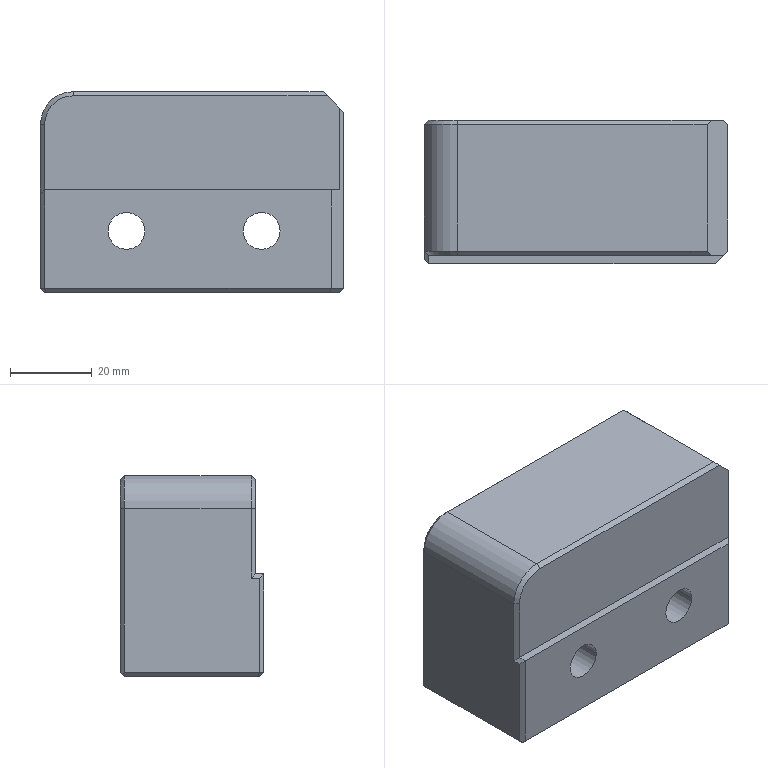Part | Creo | 1 solid | 36 faces | box 74 x 35 x 49 mm | volume 116048 mm3 | plane 25 | cylinder 9 | cone 2 | commonest cylinder face diameters 9 x4 14 x4 16 x1
STEP:
#1=CARTESIAN_POINT('',(-133.,331.995,-295.));
#2=VERTEX_POINT('',#1);
#3=CARTESIAN_POINT('',(-133.,331.995,-271.));
#4=VERTEX_POINT('',#3);
#5=CARTESIAN_POINT('',(-133.,331.995,-295.));
#6=DIRECTION('',(0.,0.,1.));
#7=VECTOR('',#6,24.);
#8=LINE('',#5,#7);
#9=EDGE_CURVE('',#2,#4,#8,.T.);
#10=ORIENTED_EDGE('',*,*,#9,.T.);
#11=CARTESIAN_POINT('',(-63.,331.995,-271.));
#12=VERTEX_POINT('',#11);
#13=CARTESIAN_POINT('',(-133.,331.995,-271.));
#14=DIRECTION('',(1.,0.,0.));
#15=VECTOR('',#14,70.);
#16=LINE('',#13,#15);
#17=EDGE_CURVE('',#4,#12,#16,.T.);
#18=ORIENTED_EDGE('',*,*,#17,.T.);
#19=CARTESIAN_POINT('',(-63.,331.995,-295.));
#20=VERTEX_POINT('',#19);
#21=CARTESIAN_POINT('',(-63.,331.995,-271.));
#22=DIRECTION('',(0.,0.,-1.));
#23=VECTOR('',#22,24.);
#24=LINE('',#21,#23);
#25=EDGE_CURVE('',#12,#20,#24,.T.);
#26=ORIENTED_EDGE('',*,*,#25,.T.);
#27=CARTESIAN_POINT('',(-63.,331.995,-295.));
#28=DIRECTION('',(-1.,0.,0.));
#29=VECTOR('',#28,70.);
#30=LINE('',#27,#29);
#31=EDGE_CURVE('',#20,#2,#30,.T.);
#32=ORIENTED_EDGE('',*,*,#31,.T.);
#33=EDGE_LOOP('',(#10,#18,#26,#32));
#34=FACE_OUTER_BOUND('',#33,.F.);
#35=CARTESIAN_POINT('',(-108.5,331.995,-281.));
#36=VERTEX_POINT('',#35);
#37=CARTESIAN_POINT('',(-117.5,331.995,-281.));
#38=VERTEX_POINT('',#37);
#39=CARTESIAN_POINT('',(-113.,331.995,-281.));
#40=DIRECTION('',(0.,1.,0.));
#41=DIRECTION('',(1.,0.,0.));
#42=AXIS2_PLACEMENT_3D('',#39,#40,#41);
#43=CIRCLE('',#42,4.5);
#44=EDGE_CURVE('',#36,#38,#43,.T.);
#45=ORIENTED_EDGE('',*,*,#44,.F.);
#46=CARTESIAN_POINT('',(-113.,331.995,-281.));
#47=DIRECTION('',(0.,1.,0.));
#48=DIRECTION('',(-1.,0.,0.));
#49=AXIS2_PLACEMENT_3D('',#46,#47,#48);
#50=CIRCLE('',#49,4.5);
#51=EDGE_CURVE('',#38,#36,#50,.T.);
#52=ORIENTED_EDGE('',*,*,#51,.F.);
#53=EDGE_LOOP('',(#45,#52));
#54=FACE_BOUND('',#53,.F.);
#55=CARTESIAN_POINT('',(-75.5,331.995,-281.));
#56=VERTEX_POINT('',#55);
#57=CARTESIAN_POINT('',(-84.5,331.995,-281.));
#58=VERTEX_POINT('',#57);
#59=CARTESIAN_POINT('',(-80.,331.995,-281.));
#60=DIRECTION('',(0.,1.,0.));
#61=DIRECTION('',(1.,0.,0.));
#62=AXIS2_PLACEMENT_3D('',#59,#60,#61);
#63=CIRCLE('',#62,4.5);
#64=EDGE_CURVE('',#56,#58,#63,.T.);
#65=ORIENTED_EDGE('',*,*,#64,.F.);
#66=CARTESIAN_POINT('',(-80.,331.995,-281.));
#67=DIRECTION('',(0.,1.,0.));
#68=DIRECTION('',(-1.,0.,0.));
#69=AXIS2_PLACEMENT_3D('',#66,#67,#68);
#70=CIRCLE('',#69,4.5);
#71=EDGE_CURVE('',#58,#56,#70,.T.);
#72=ORIENTED_EDGE('',*,*,#71,.F.);
#73=EDGE_LOOP('',(#65,#72));
#74=FACE_BOUND('',#73,.F.);
#75=CARTESIAN_POINT('',(-162.,331.995,-10.));
#76=DIRECTION('',(0.,1.,0.));
#77=DIRECTION('',(-1.,0.,0.));
#78=AXIS2_PLACEMENT_3D('',#75,#76,#77);
#79=PLANE('',#78);
#80=ADVANCED_FACE('',(#34,#54,#74),#79,.F.);
#81=ORIENTED_EDGE('',*,*,#64,.T.);
#82=CARTESIAN_POINT('',(-84.5,357.995,-281.));
#83=VERTEX_POINT('',#82);
#84=CARTESIAN_POINT('',(-84.5,331.995,-281.));
#85=DIRECTION('',(0.,1.,0.));
#86=VECTOR('',#85,26.);
#87=LINE('',#84,#86);
#88=EDGE_CURVE('',#58,#83,#87,.T.);
#89=ORIENTED_EDGE('',*,*,#88,.T.);
#90=CARTESIAN_POINT('',(-75.5,357.995,-281.));
#91=VERTEX_POINT('',#90);
#92=CARTESIAN_POINT('',(-80.,357.995,-281.));
#93=DIRECTION('',(0.,-1.,0.));
#94=DIRECTION('',(-1.,0.,0.));
#95=AXIS2_PLACEMENT_3D('',#92,#93,#94);
#96=CIRCLE('',#95,4.5);
#97=EDGE_CURVE('',#83,#91,#96,.T.);
#98=ORIENTED_EDGE('',*,*,#97,.T.);
#99=CARTESIAN_POINT('',(-75.5,331.995,-281.));
#100=DIRECTION('',(0.,1.,0.));
#101=VECTOR('',#100,26.);
#102=LINE('',#99,#101);
#103=EDGE_CURVE('',#56,#91,#102,.T.);
#104=ORIENTED_EDGE('',*,*,#103,.F.);
#105=EDGE_LOOP('',(#81,#89,#98,#104));
#106=FACE_OUTER_BOUND('',#105,.F.);
#107=CARTESIAN_POINT('',(-80.,366.995,-281.));
#108=DIRECTION('',(0.,1.,0.));
#109=DIRECTION('',(-1.,0.,0.));
#110=AXIS2_PLACEMENT_3D('',#107,#108,#109);
#111=CYLINDRICAL_SURFACE('',#110,4.5);
#112=ADVANCED_FACE('',(#106),#111,.F.);
#113=ORIENTED_EDGE('',*,*,#71,.T.);
#114=ORIENTED_EDGE('',*,*,#103,.T.);
#115=CARTESIAN_POINT('',(-80.,357.995,-281.));
#116=DIRECTION('',(0.,-1.,0.));
#117=DIRECTION('',(1.,0.,0.));
#118=AXIS2_PLACEMENT_3D('',#115,#116,#117);
#119=CIRCLE('',#118,4.5);
#120=EDGE_CURVE('',#91,#83,#119,.T.);
#121=ORIENTED_EDGE('',*,*,#120,.T.);
#122=ORIENTED_EDGE('',*,*,#88,.F.);
#123=EDGE_LOOP('',(#113,#114,#121,#122));
#124=FACE_OUTER_BOUND('',#123,.F.);
#125=CARTESIAN_POINT('',(-80.,366.995,-281.));
#126=DIRECTION('',(0.,1.,0.));
#127=DIRECTION('',(-1.,0.,0.));
#128=AXIS2_PLACEMENT_3D('',#125,#126,#127);
#129=CYLINDRICAL_SURFACE('',#128,4.5);
#130=ADVANCED_FACE('',(#124),#129,.F.);
#131=CARTESIAN_POINT('',(-73.,357.995,-281.));
#132=VERTEX_POINT('',#131);
#133=CARTESIAN_POINT('',(-87.,357.995,-281.));
#134=VERTEX_POINT('',#133);
#135=CARTESIAN_POINT('',(-80.,357.995,-281.));
#136=DIRECTION('',(0.,1.,0.));
#137=DIRECTION('',(1.,0.,0.));
#138=AXIS2_PLACEMENT_3D('',#135,#136,#137);
#139=CIRCLE('',#138,7.);
#140=EDGE_CURVE('',#132,#134,#139,.T.);
#141=ORIENTED_EDGE('',*,*,#140,.F.);
#142=CARTESIAN_POINT('',(-80.,357.995,-281.));
#143=DIRECTION('',(0.,1.,0.));
#144=DIRECTION('',(-1.,0.,0.));
#145=AXIS2_PLACEMENT_3D('',#142,#143,#144);
#146=CIRCLE('',#145,7.);
#147=EDGE_CURVE('',#134,#132,#146,.T.);
#148=ORIENTED_EDGE('',*,*,#147,.F.);
#149=EDGE_LOOP('',(#141,#148));
#150=FACE_OUTER_BOUND('',#149,.F.);
#151=ORIENTED_EDGE('',*,*,#120,.F.);
#152=ORIENTED_EDGE('',*,*,#97,.F.);
#153=EDGE_LOOP('',(#151,#152));
#154=FACE_BOUND('',#153,.F.);
#155=CARTESIAN_POINT('',(-80.,357.995,-288.));
#156=DIRECTION('',(0.,-1.,0.));
#157=DIRECTION('',(1.,0.,0.));
#158=AXIS2_PLACEMENT_3D('',#155,#156,#157);
#159=PLANE('',#158);
#160=ADVANCED_FACE('',(#150,#154),#159,.F.);
#161=ORIENTED_EDGE('',*,*,#140,.T.);
#162=CARTESIAN_POINT('',(-87.,366.995,-281.));
#163=VERTEX_POINT('',#162);
#164=CARTESIAN_POINT('',(-87.,357.995,-281.));
#165=DIRECTION('',(0.,1.,0.));
#166=VECTOR('',#165,9.);
#167=LINE('',#164,#166);
#168=EDGE_CURVE('',#134,#163,#167,.T.);
#169=ORIENTED_EDGE('',*,*,#168,.T.);
#170=CARTESIAN_POINT('',(-73.,366.995,-281.));
#171=VERTEX_POINT('',#170);
#172=CARTESIAN_POINT('',(-80.,366.995,-281.));
#173=DIRECTION('',(0.,-1.,0.));
#174=DIRECTION('',(-1.,0.,0.));
#175=AXIS2_PLACEMENT_3D('',#172,#173,#174);
#176=CIRCLE('',#175,7.);
#177=EDGE_CURVE('',#163,#171,#176,.T.);
#178=ORIENTED_EDGE('',*,*,#177,.T.);
#179=CARTESIAN_POINT('',(-73.,357.995,-281.));
#180=DIRECTION('',(0.,1.,0.));
#181=VECTOR('',#180,9.);
#182=LINE('',#179,#181);
#183=EDGE_CURVE('',#132,#171,#182,.T.);
#184=ORIENTED_EDGE('',*,*,#183,.F.);
#185=EDGE_LOOP('',(#161,#169,#178,#184));
#186=FACE_OUTER_BOUND('',#185,.F.);
#187=CARTESIAN_POINT('',(-80.,366.995,-281.));
#188=DIRECTION('',(0.,1.,0.));
#189=DIRECTION('',(-1.,0.,0.));
#190=AXIS2_PLACEMENT_3D('',#187,#188,#189);
#191=CYLINDRICAL_SURFACE('',#190,7.);
#192=ADVANCED_FACE('',(#186),#191,.F.);
#193=ORIENTED_EDGE('',*,*,#147,.T.);
#194=ORIENTED_EDGE('',*,*,#183,.T.);
#195=CARTESIAN_POINT('',(-80.,366.995,-281.));
#196=DIRECTION('',(0.,-1.,0.));
#197=DIRECTION('',(1.,0.,0.));
#198=AXIS2_PLACEMENT_3D('',#195,#196,#197);
#199=CIRCLE('',#198,7.);
#200=EDGE_CURVE('',#171,#163,#199,.T.);
#201=ORIENTED_EDGE('',*,*,#200,.T.);
#202=ORIENTED_EDGE('',*,*,#168,.F.);
#203=EDGE_LOOP('',(#193,#194,#201,#202));
#204=FACE_OUTER_BOUND('',#203,.F.);
#205=CARTESIAN_POINT('',(-80.,366.995,-281.));
#206=DIRECTION('',(0.,1.,0.));
#207=DIRECTION('',(-1.,0.,0.));
#208=AXIS2_PLACEMENT_3D('',#205,#206,#207);
#209=CYLINDRICAL_SURFACE('',#208,7.);
#210=ADVANCED_FACE('',(#204),#209,.F.);
#211=CARTESIAN_POINT('',(-64.,366.995,-248.));
#212=VERTEX_POINT('',#211);
#213=CARTESIAN_POINT('',(-126.,366.995,-248.));
#214=VERTEX_POINT('',#213);
#215=CARTESIAN_POINT('',(-64.,366.995,-248.));
#216=DIRECTION('',(-1.,0.,0.));
#217=VECTOR('',#216,62.);
#218=LINE('',#215,#217);
#219=EDGE_CURVE('',#212,#214,#218,.T.);
#220=ORIENTED_EDGE('',*,*,#219,.T.);
#221=CARTESIAN_POINT('',(-133.,366.995,-255.));
#222=VERTEX_POINT('',#221);
#223=CARTESIAN_POINT('',(-126.,366.995,-255.));
#224=DIRECTION('',(0.,1.,0.));
#225=DIRECTION('',(-1.,0.,0.));
#226=AXIS2_PLACEMENT_3D('',#223,#224,#225);
#227=CIRCLE('',#226,7.);
#228=EDGE_CURVE('',#222,#214,#227,.T.);
#229=ORIENTED_EDGE('',*,*,#228,.F.);
#230=CARTESIAN_POINT('',(-133.,366.995,-295.));
#231=VERTEX_POINT('',#230);
#232=CARTESIAN_POINT('',(-133.,366.995,-255.));
#233=DIRECTION('',(0.,0.,-1.));
#234=VECTOR('',#233,40.);
#235=LINE('',#232,#234);
#236=EDGE_CURVE('',#222,#231,#235,.T.);
#237=ORIENTED_EDGE('',*,*,#236,.T.);
#238=CARTESIAN_POINT('',(-61.,366.995,-295.));
#239=VERTEX_POINT('',#238);
#240=CARTESIAN_POINT('',(-133.,366.995,-295.));
#241=DIRECTION('',(1.,0.,0.));
#242=VECTOR('',#241,72.);
#243=LINE('',#240,#242);
#244=EDGE_CURVE('',#231,#239,#243,.T.);
#245=ORIENTED_EDGE('',*,*,#244,.T.);
#246=CARTESIAN_POINT('',(-61.,366.995,-251.));
#247=VERTEX_POINT('',#246);
#248=CARTESIAN_POINT('',(-61.,366.995,-295.));
#249=DIRECTION('',(0.,0.,1.));
#250=VECTOR('',#249,44.);
#251=LINE('',#248,#250);
#252=EDGE_CURVE('',#239,#247,#251,.T.);
#253=ORIENTED_EDGE('',*,*,#252,.T.);
#254=CARTESIAN_POINT('',(-64.,366.995,-248.));
#255=DIRECTION('',(0.7071,0.,-0.7071));
#256=VECTOR('',#255,4.243);
#257=LINE('',#254,#256);
#258=EDGE_CURVE('',#212,#247,#257,.T.);
#259=ORIENTED_EDGE('',*,*,#258,.F.);
#260=EDGE_LOOP('',(#220,#229,#237,#245,#253,#259));
#261=FACE_OUTER_BOUND('',#260,.F.);
#262=CARTESIAN_POINT('',(-106.,366.995,-281.));
#263=VERTEX_POINT('',#262);
#264=CARTESIAN_POINT('',(-120.,366.995,-281.));
#265=VERTEX_POINT('',#264);
#266=CARTESIAN_POINT('',(-113.,366.995,-281.));
#267=DIRECTION('',(0.,-1.,0.));
#268=DIRECTION('',(1.,0.,0.));
#269=AXIS2_PLACEMENT_3D('',#266,#267,#268);
#270=CIRCLE('',#269,7.);
#271=EDGE_CURVE('',#263,#265,#270,.T.);
#272=ORIENTED_EDGE('',*,*,#271,.F.);
#273=CARTESIAN_POINT('',(-113.,366.995,-281.));
#274=DIRECTION('',(0.,-1.,0.));
#275=DIRECTION('',(-1.,0.,0.));
#276=AXIS2_PLACEMENT_3D('',#273,#274,#275);
#277=CIRCLE('',#276,7.);
#278=EDGE_CURVE('',#265,#263,#277,.T.);
#279=ORIENTED_EDGE('',*,*,#278,.F.);
#280=EDGE_LOOP('',(#272,#279));
#281=FACE_BOUND('',#280,.F.);
#282=ORIENTED_EDGE('',*,*,#200,.F.);
#283=ORIENTED_EDGE('',*,*,#177,.F.);
#284=EDGE_LOOP('',(#282,#283));
#285=FACE_BOUND('',#284,.F.);
#286=CARTESIAN_POINT('',(-162.,366.995,-10.));
#287=DIRECTION('',(0.,1.,0.));
#288=DIRECTION('',(-1.,0.,0.));
#289=AXIS2_PLACEMENT_3D('',#286,#287,#288);
#290=PLANE('',#289);
#291=ADVANCED_FACE('',(#261,#281,#285),#290,.T.);
#292=CARTESIAN_POINT('',(-120.,357.995,-281.));
#293=VERTEX_POINT('',#292);
#294=CARTESIAN_POINT('',(-106.,357.995,-281.));
#295=VERTEX_POINT('',#294);
#296=CARTESIAN_POINT('',(-113.,357.995,-281.));
#297=DIRECTION('',(0.,1.,0.));
#298=DIRECTION('',(-1.,0.,0.));
#299=AXIS2_PLACEMENT_3D('',#296,#297,#298);
#300=CIRCLE('',#299,7.);
#301=EDGE_CURVE('',#293,#295,#300,.T.);
#302=ORIENTED_EDGE('',*,*,#301,.T.);
#303=CARTESIAN_POINT('',(-106.,357.995,-281.));
#304=DIRECTION('',(0.,1.,0.));
#305=VECTOR('',#304,9.);
#306=LINE('',#303,#305);
#307=EDGE_CURVE('',#295,#263,#306,.T.);
#308=ORIENTED_EDGE('',*,*,#307,.T.);
#309=ORIENTED_EDGE('',*,*,#271,.T.);
#310=CARTESIAN_POINT('',(-120.,357.995,-281.));
#311=DIRECTION('',(0.,1.,0.));
#312=VECTOR('',#311,9.);
#313=LINE('',#310,#312);
#314=EDGE_CURVE('',#293,#265,#313,.T.);
#315=ORIENTED_EDGE('',*,*,#314,.F.);
#316=EDGE_LOOP('',(#302,#308,#309,#315));
#317=FACE_OUTER_BOUND('',#316,.F.);
#318=CARTESIAN_POINT('',(-113.,366.995,-281.));
#319=DIRECTION('',(0.,1.,0.));
#320=DIRECTION('',(-1.,0.,0.));
#321=AXIS2_PLACEMENT_3D('',#318,#319,#320);
#322=CYLINDRICAL_SURFACE('',#321,7.);
#323=ADVANCED_FACE('',(#317),#322,.F.);
#324=CARTESIAN_POINT('',(-113.,357.995,-281.));
#325=DIRECTION('',(0.,1.,0.));
#326=DIRECTION('',(1.,0.,0.));
#327=AXIS2_PLACEMENT_3D('',#324,#325,#326);
#328=CIRCLE('',#327,7.);
#329=EDGE_CURVE('',#295,#293,#328,.T.);
#330=ORIENTED_EDGE('',*,*,#329,.F.);
#331=ORIENTED_EDGE('',*,*,#301,.F.);
#332=EDGE_LOOP('',(#330,#331));
#333=FACE_OUTER_BOUND('',#332,.F.);
#334=CARTESIAN_POINT('',(-108.5,357.995,-281.));
#335=VERTEX_POINT('',#334);
#336=CARTESIAN_POINT('',(-117.5,357.995,-281.));
#337=VERTEX_POINT('',#336);
#338=CARTESIAN_POINT('',(-113.,357.995,-281.));
#339=DIRECTION('',(0.,-1.,0.));
#340=DIRECTION('',(1.,0.,0.));
#341=AXIS2_PLACEMENT_3D('',#338,#339,#340);
#342=CIRCLE('',#341,4.5);
#343=EDGE_CURVE('',#335,#337,#342,.T.);
#344=ORIENTED_EDGE('',*,*,#343,.F.);
#345=CARTESIAN_POINT('',(-113.,357.995,-281.));
#346=DIRECTION('',(0.,-1.,0.));
#347=DIRECTION('',(-1.,0.,0.));
#348=AXIS2_PLACEMENT_3D('',#345,#346,#347);
#349=CIRCLE('',#348,4.5);
#350=EDGE_CURVE('',#337,#335,#349,.T.);
#351=ORIENTED_EDGE('',*,*,#350,.F.);
#352=EDGE_LOOP('',(#344,#351));
#353=FACE_BOUND('',#352,.F.);
#354=CARTESIAN_POINT('',(-113.,357.995,-288.));
#355=DIRECTION('',(0.,-1.,0.));
#356=DIRECTION('',(1.,0.,0.));
#357=AXIS2_PLACEMENT_3D('',#354,#355,#356);
#358=PLANE('',#357);
#359=ADVANCED_FACE('',(#333,#353),#358,.F.);
#360=ORIENTED_EDGE('',*,*,#51,.T.);
#361=CARTESIAN_POINT('',(-108.5,331.995,-281.));
#362=DIRECTION('',(0.,1.,0.));
#363=VECTOR('',#362,26.);
#364=LINE('',#361,#363);
#365=EDGE_CURVE('',#36,#335,#364,.T.);
#366=ORIENTED_EDGE('',*,*,#365,.T.);
#367=ORIENTED_EDGE('',*,*,#343,.T.);
#368=CARTESIAN_POINT('',(-117.5,331.995,-281.));
#369=DIRECTION('',(0.,1.,0.));
#370=VECTOR('',#369,26.);
#371=LINE('',#368,#370);
#372=EDGE_CURVE('',#38,#337,#371,.T.);
#373=ORIENTED_EDGE('',*,*,#372,.F.);
#374=EDGE_LOOP('',(#360,#366,#367,#373));
#375=FACE_OUTER_BOUND('',#374,.F.);
#376=CARTESIAN_POINT('',(-113.,366.995,-281.));
#377=DIRECTION('',(0.,1.,0.));
#378=DIRECTION('',(-1.,0.,0.));
#379=AXIS2_PLACEMENT_3D('',#376,#377,#378);
#380=CYLINDRICAL_SURFACE('',#379,4.5);
#381=ADVANCED_FACE('',(#375),#380,.F.);
#382=ORIENTED_EDGE('',*,*,#44,.T.);
#383=ORIENTED_EDGE('',*,*,#372,.T.);
#384=ORIENTED_EDGE('',*,*,#350,.T.);
#385=ORIENTED_EDGE('',*,*,#365,.F.);
#386=EDGE_LOOP('',(#382,#383,#384,#385));
#387=FACE_OUTER_BOUND('',#386,.F.);
#388=CARTESIAN_POINT('',(-113.,366.995,-281.));
#389=DIRECTION('',(0.,1.,0.));
#390=DIRECTION('',(-1.,0.,0.));
#391=AXIS2_PLACEMENT_3D('',#388,#389,#390);
#392=CYLINDRICAL_SURFACE('',#391,4.5);
#393=ADVANCED_FACE('',(#387),#392,.F.);
#394=ORIENTED_EDGE('',*,*,#329,.T.);
#395=ORIENTED_EDGE('',*,*,#314,.T.);
#396=ORIENTED_EDGE('',*,*,#278,.T.);
#397=ORIENTED_EDGE('',*,*,#307,.F.);
#398=EDGE_LOOP('',(#394,#395,#396,#397));
#399=FACE_OUTER_BOUND('',#398,.F.);
#400=CARTESIAN_POINT('',(-113.,366.995,-281.));
#401=DIRECTION('',(0.,1.,0.));
#402=DIRECTION('',(-1.,0.,0.));
#403=AXIS2_PLACEMENT_3D('',#400,#401,#402);
#404=CYLINDRICAL_SURFACE('',#403,7.);
#405=ADVANCED_FACE('',(#399),#404,.F.);
#406=CARTESIAN_POINT('',(-65.,365.995,-247.));
#407=VERTEX_POINT('',#406);
#408=CARTESIAN_POINT('',(-126.,365.995,-247.));
#409=VERTEX_POINT('',#408);
#410=CARTESIAN_POINT('',(-65.,365.995,-247.));
#411=DIRECTION('',(-1.,0.,0.));
#412=VECTOR('',#411,61.);
#413=LINE('',#410,#412);
#414=EDGE_CURVE('',#407,#409,#413,.T.);
#415=ORIENTED_EDGE('',*,*,#414,.T.);
#416=CARTESIAN_POINT('',(-126.,365.995,-247.));
#417=DIRECTION('',(0.,0.7071,-0.7071));
#418=VECTOR('',#417,1.414);
#419=LINE('',#416,#418);
#420=EDGE_CURVE('',#409,#214,#419,.T.);
#421=ORIENTED_EDGE('',*,*,#420,.T.);
#422=ORIENTED_EDGE('',*,*,#219,.F.);
#423=CARTESIAN_POINT('',(-64.,366.995,-248.));
#424=DIRECTION('',(-0.5774,-0.5774,0.5774));
#425=VECTOR('',#424,1.732);
#426=LINE('',#423,#425);
#427=EDGE_CURVE('',#212,#407,#426,.T.);
#428=ORIENTED_EDGE('',*,*,#427,.T.);
#429=EDGE_LOOP('',(#415,#421,#422,#428));
#430=FACE_OUTER_BOUND('',#429,.F.);
#431=CARTESIAN_POINT('',(-112.,366.495,-247.5));
#432=DIRECTION('',(0.,0.7071,0.7071));
#433=DIRECTION('',(0.,-0.7071,0.7071));
#434=AXIS2_PLACEMENT_3D('',#431,#432,#433);
#435=PLANE('',#434);
#436=ADVANCED_FACE('',(#430),#435,.T.);
#437=CARTESIAN_POINT('',(-65.,334.995,-247.));
#438=VERTEX_POINT('',#437);
#439=CARTESIAN_POINT('',(-126.,334.995,-247.));
#440=VERTEX_POINT('',#439);
#441=CARTESIAN_POINT('',(-65.,334.995,-247.));
#442=DIRECTION('',(-1.,0.,0.));
#443=VECTOR('',#442,61.);
#444=LINE('',#441,#443);
#445=EDGE_CURVE('',#438,#440,#444,.T.);
#446=ORIENTED_EDGE('',*,*,#445,.T.);
#447=CARTESIAN_POINT('',(-126.,334.995,-247.));
#448=DIRECTION('',(0.,1.,0.));
#449=VECTOR('',#448,31.);
#450=LINE('',#447,#449);
#451=EDGE_CURVE('',#440,#409,#450,.T.);
#452=ORIENTED_EDGE('',*,*,#451,.T.);
#453=ORIENTED_EDGE('',*,*,#414,.F.);
#454=CARTESIAN_POINT('',(-65.,365.995,-247.));
#455=DIRECTION('',(0.,-1.,0.));
#456=VECTOR('',#455,31.);
#457=LINE('',#454,#456);
#458=EDGE_CURVE('',#407,#438,#457,.T.);
#459=ORIENTED_EDGE('',*,*,#458,.T.);
#460=EDGE_LOOP('',(#446,#452,#453,#459));
#461=FACE_OUTER_BOUND('',#460,.F.);
#462=CARTESIAN_POINT('',(-135.,331.995,-247.));
#463=DIRECTION('',(0.,0.,1.));
#464=DIRECTION('',(1.,0.,0.));
#465=AXIS2_PLACEMENT_3D('',#462,#463,#464);
#466=PLANE('',#465);
#467=ADVANCED_FACE('',(#461),#466,.T.);
#468=CARTESIAN_POINT('',(-64.,333.995,-248.));
#469=VERTEX_POINT('',#468);
#470=CARTESIAN_POINT('',(-126.,333.995,-248.));
#471=VERTEX_POINT('',#470);
#472=CARTESIAN_POINT('',(-64.,333.995,-248.));
#473=DIRECTION('',(-1.,0.,0.));
#474=VECTOR('',#473,62.);
#475=LINE('',#472,#474);
#476=EDGE_CURVE('',#469,#471,#475,.T.);
#477=ORIENTED_EDGE('',*,*,#476,.T.);
#478=CARTESIAN_POINT('',(-126.,333.995,-248.));
#479=DIRECTION('',(0.,0.7071,0.7071));
#480=VECTOR('',#479,1.414);
#481=LINE('',#478,#480);
#482=EDGE_CURVE('',#471,#440,#481,.T.);
#483=ORIENTED_EDGE('',*,*,#482,.T.);
#484=ORIENTED_EDGE('',*,*,#445,.F.);
#485=CARTESIAN_POINT('',(-65.,334.995,-247.));
#486=DIRECTION('',(0.5774,-0.5774,-0.5774));
#487=VECTOR('',#486,1.732);
#488=LINE('',#485,#487);
#489=EDGE_CURVE('',#438,#469,#488,.T.);
#490=ORIENTED_EDGE('',*,*,#489,.T.);
#491=EDGE_LOOP('',(#477,#483,#484,#490));
#492=FACE_OUTER_BOUND('',#491,.F.);
#493=CARTESIAN_POINT('',(-112.,334.495,-247.5));
#494=DIRECTION('',(0.,-0.7071,0.7071));
#495=DIRECTION('',(0.,-0.7071,-0.7071));
#496=AXIS2_PLACEMENT_3D('',#493,#494,#495);
#497=PLANE('',#496);
#498=ADVANCED_FACE('',(#492),#497,.T.);
#499=CARTESIAN_POINT('',(-61.,333.995,-251.));
#500=VERTEX_POINT('',#499);
#501=CARTESIAN_POINT('',(-61.,333.995,-271.));
#502=VERTEX_POINT('',#501);
#503=CARTESIAN_POINT('',(-61.,333.995,-251.));
#504=DIRECTION('',(0.,0.,-1.));
#505=VECTOR('',#504,20.);
#506=LINE('',#503,#505);
#507=EDGE_CURVE('',#500,#502,#506,.T.);
#508=ORIENTED_EDGE('',*,*,#507,.T.);
#509=CARTESIAN_POINT('',(-133.,333.995,-271.));
#510=VERTEX_POINT('',#509);
#511=CARTESIAN_POINT('',(-61.,333.995,-271.));
#512=DIRECTION('',(-1.,0.,0.));
#513=VECTOR('',#512,72.);
#514=LINE('',#511,#513);
#515=EDGE_CURVE('',#502,#510,#514,.T.);
#516=ORIENTED_EDGE('',*,*,#515,.T.);
#517=CARTESIAN_POINT('',(-133.,333.995,-255.));
#518=VERTEX_POINT('',#517);
#519=CARTESIAN_POINT('',(-133.,333.995,-255.));
#520=DIRECTION('',(0.,0.,-1.));
#521=VECTOR('',#520,16.);
#522=LINE('',#519,#521);
#523=EDGE_CURVE('',#518,#510,#522,.T.);
#524=ORIENTED_EDGE('',*,*,#523,.F.);
#525=CARTESIAN_POINT('',(-126.,333.995,-255.));
#526=DIRECTION('',(0.,-1.,0.));
#527=DIRECTION('',(0.,0.,1.));
#528=AXIS2_PLACEMENT_3D('',#525,#526,#527);
#529=CIRCLE('',#528,7.);
#530=EDGE_CURVE('',#471,#518,#529,.T.);
#531=ORIENTED_EDGE('',*,*,#530,.F.);
#532=ORIENTED_EDGE('',*,*,#476,.F.);
#533=CARTESIAN_POINT('',(-61.,333.995,-251.));
#534=DIRECTION('',(-0.7071,0.,0.7071));
#535=VECTOR('',#534,4.243);
#536=LINE('',#533,#535);
#537=EDGE_CURVE('',#500,#469,#536,.T.);
#538=ORIENTED_EDGE('',*,*,#537,.F.);
#539=EDGE_LOOP('',(#508,#516,#524,#531,#532,#538));
#540=FACE_OUTER_BOUND('',#539,.F.);
#541=CARTESIAN_POINT('',(-162.,333.995,-10.));
#542=DIRECTION('',(0.,-1.,0.));
#543=DIRECTION('',(1.,0.,0.));
#544=AXIS2_PLACEMENT_3D('',#541,#542,#543);
#545=PLANE('',#544);
#546=ADVANCED_FACE('',(#540),#545,.T.);
#547=ORIENTED_EDGE('',*,*,#25,.F.);
#548=CARTESIAN_POINT('',(-63.,331.995,-271.));
#549=DIRECTION('',(0.7071,0.7071,0.));
#550=VECTOR('',#549,2.828);
#551=LINE('',#548,#550);
#552=EDGE_CURVE('',#12,#502,#551,.T.);
#553=ORIENTED_EDGE('',*,*,#552,.T.);
#554=ORIENTED_EDGE('',*,*,#507,.F.);
#555=CARTESIAN_POINT('',(-60.,334.995,-252.));
#556=VERTEX_POINT('',#555);
#557=CARTESIAN_POINT('',(-61.,333.995,-251.));
#558=DIRECTION('',(0.5774,0.5774,-0.5774));
#559=VECTOR('',#558,1.732);
#560=LINE('',#557,#559);
#561=EDGE_CURVE('',#500,#556,#560,.T.);
#562=ORIENTED_EDGE('',*,*,#561,.T.);
#563=CARTESIAN_POINT('',(-60.,334.995,-295.));
#564=VERTEX_POINT('',#563);
#565=CARTESIAN_POINT('',(-60.,334.995,-295.));
#566=DIRECTION('',(0.,0.,1.));
#567=VECTOR('',#566,43.);
#568=LINE('',#565,#567);
#569=EDGE_CURVE('',#564,#556,#568,.T.);
#570=ORIENTED_EDGE('',*,*,#569,.F.);
#571=CARTESIAN_POINT('',(-60.,334.995,-295.));
#572=DIRECTION('',(-0.7071,-0.7071,0.));
#573=VECTOR('',#572,4.243);
#574=LINE('',#571,#573);
#575=EDGE_CURVE('',#564,#20,#574,.T.);
#576=ORIENTED_EDGE('',*,*,#575,.T.);
#577=EDGE_LOOP('',(#547,#553,#554,#562,#570,#576));
#578=FACE_OUTER_BOUND('',#577,.F.);
#579=CARTESIAN_POINT('',(-63.,331.995,-10.));
#580=DIRECTION('',(0.7071,-0.7071,0.));
#581=DIRECTION('',(0.,0.,1.));
#582=AXIS2_PLACEMENT_3D('',#579,#580,#581);
#583=PLANE('',#582);
#584=ADVANCED_FACE('',(#578),#583,.T.);
#585=ORIENTED_EDGE('',*,*,#17,.F.);
#586=CARTESIAN_POINT('',(-133.,333.995,-271.));
#587=DIRECTION('',(0.,-1.,0.));
#588=VECTOR('',#587,2.);
#589=LINE('',#586,#588);
#590=EDGE_CURVE('',#510,#4,#589,.T.);
#591=ORIENTED_EDGE('',*,*,#590,.F.);
#592=ORIENTED_EDGE('',*,*,#515,.F.);
#593=ORIENTED_EDGE('',*,*,#552,.F.);
#594=EDGE_LOOP('',(#585,#591,#592,#593));
#595=FACE_OUTER_BOUND('',#594,.F.);
#596=CARTESIAN_POINT('',(-227.861,331.995,-271.));
#597=DIRECTION('',(0.,0.,-1.));
#598=DIRECTION('',(1.,0.,0.));
#599=AXIS2_PLACEMENT_3D('',#596,#597,#598);
#600=PLANE('',#599);
#601=ADVANCED_FACE('',(#595),#600,.F.);
#602=ORIENTED_EDGE('',*,*,#590,.T.);
#603=CARTESIAN_POINT('',(-134.,332.995,-272.));
#604=VERTEX_POINT('',#603);
#605=CARTESIAN_POINT('',(-134.,332.995,-272.));
#606=DIRECTION('',(0.5774,-0.5774,0.5774));
#607=VECTOR('',#606,1.732);
#608=LINE('',#605,#607);
#609=EDGE_CURVE('',#604,#4,#608,.T.);
#610=ORIENTED_EDGE('',*,*,#609,.F.);
#611=CARTESIAN_POINT('',(-134.,334.995,-272.));
#612=VERTEX_POINT('',#611);
#613=CARTESIAN_POINT('',(-134.,334.995,-272.));
#614=DIRECTION('',(0.,-1.,0.));
#615=VECTOR('',#614,2.);
#616=LINE('',#613,#615);
#617=EDGE_CURVE('',#612,#604,#616,.T.);
#618=ORIENTED_EDGE('',*,*,#617,.F.);
#619=CARTESIAN_POINT('',(-134.,334.995,-272.));
#620=DIRECTION('',(0.5774,-0.5774,0.5774));
#621=VECTOR('',#620,1.732);
#622=LINE('',#619,#621);
#623=EDGE_CURVE('',#612,#510,#622,.T.);
#624=ORIENTED_EDGE('',*,*,#623,.T.);
#625=EDGE_LOOP('',(#602,#610,#618,#624));
#626=FACE_OUTER_BOUND('',#625,.F.);
#627=CARTESIAN_POINT('',(-133.5,333.495,-271.5));
#628=DIRECTION('',(-0.7071,0.,0.7071));
#629=DIRECTION('',(0.7071,0.,0.7071));
#630=AXIS2_PLACEMENT_3D('',#627,#628,#629);
#631=PLANE('',#630);
#632=ADVANCED_FACE('',(#626),#631,.T.);
#633=CARTESIAN_POINT('',(-134.,332.995,-295.));
#634=VERTEX_POINT('',#633);
#635=CARTESIAN_POINT('',(-134.,332.995,-295.));
#636=DIRECTION('',(0.,0.,1.));
#637=VECTOR('',#636,23.);
#638=LINE('',#635,#637);
#639=EDGE_CURVE('',#634,#604,#638,.T.);
#640=ORIENTED_EDGE('',*,*,#639,.T.);
#641=ORIENTED_EDGE('',*,*,#609,.T.);
#642=ORIENTED_EDGE('',*,*,#9,.F.);
#643=CARTESIAN_POINT('',(-133.,331.995,-295.));
#644=DIRECTION('',(-0.7071,0.7071,0.));
#645=VECTOR('',#644,1.414);
#646=LINE('',#643,#645);
#647=EDGE_CURVE('',#2,#634,#646,.T.);
#648=ORIENTED_EDGE('',*,*,#647,.T.);
#649=EDGE_LOOP('',(#640,#641,#642,#648));
#650=FACE_OUTER_BOUND('',#649,.F.);
#651=CARTESIAN_POINT('',(-133.5,332.495,-289.));
#652=DIRECTION('',(-0.7071,-0.7071,0.));
#653=DIRECTION('',(-0.7071,0.7071,0.));
#654=AXIS2_PLACEMENT_3D('',#651,#652,#653);
#655=PLANE('',#654);
#656=ADVANCED_FACE('',(#650),#655,.T.);
#657=CARTESIAN_POINT('',(-134.,365.995,-255.));
#658=VERTEX_POINT('',#657);
#659=CARTESIAN_POINT('',(-134.,365.995,-295.));
#660=VERTEX_POINT('',#659);
#661=CARTESIAN_POINT('',(-134.,365.995,-255.));
#662=DIRECTION('',(0.,0.,-1.));
#663=VECTOR('',#662,40.);
#664=LINE('',#661,#663);
#665=EDGE_CURVE('',#658,#660,#664,.T.);
#666=ORIENTED_EDGE('',*,*,#665,.F.);
#667=CARTESIAN_POINT('',(-134.,334.995,-255.));
#668=VERTEX_POINT('',#667);
#669=CARTESIAN_POINT('',(-134.,365.995,-255.));
#670=DIRECTION('',(0.,-1.,0.));
#671=VECTOR('',#670,31.);
#672=LINE('',#669,#671);
#673=EDGE_CURVE('',#658,#668,#672,.T.);
#674=ORIENTED_EDGE('',*,*,#673,.T.);
#675=CARTESIAN_POINT('',(-134.,334.995,-255.));
#676=DIRECTION('',(0.,0.,-1.));
#677=VECTOR('',#676,17.);
#678=LINE('',#675,#677);
#679=EDGE_CURVE('',#668,#612,#678,.T.);
#680=ORIENTED_EDGE('',*,*,#679,.T.);
#681=ORIENTED_EDGE('',*,*,#617,.T.);
#682=ORIENTED_EDGE('',*,*,#639,.F.);
#683=CARTESIAN_POINT('',(-134.,332.995,-295.));
#684=DIRECTION('',(0.,1.,0.));
#685=VECTOR('',#684,33.);
#686=LINE('',#683,#685);
#687=EDGE_CURVE('',#634,#660,#686,.T.);
#688=ORIENTED_EDGE('',*,*,#687,.T.);
#689=EDGE_LOOP('',(#666,#674,#680,#681,#682,#688));
#690=FACE_OUTER_BOUND('',#689,.F.);
#691=CARTESIAN_POINT('',(-134.,331.995,-326.));
#692=DIRECTION('',(-1.,0.,0.));
#693=DIRECTION('',(0.,0.,1.));
#694=AXIS2_PLACEMENT_3D('',#691,#692,#693);
#695=PLANE('',#694);
#696=ADVANCED_FACE('',(#690),#695,.T.);
#697=CARTESIAN_POINT('',(-133.5,366.495,-295.5));
#698=VERTEX_POINT('',#697);
#699=CARTESIAN_POINT('',(-133.5,366.495,-295.5));
#700=DIRECTION('',(0.5774,0.5774,0.5774));
#701=VECTOR('',#700,0.866);
#702=LINE('',#699,#701);
#703=EDGE_CURVE('',#698,#231,#702,.T.);
#704=ORIENTED_EDGE('',*,*,#703,.T.);
#705=ORIENTED_EDGE('',*,*,#236,.F.);
#706=CARTESIAN_POINT('',(-133.,366.995,-255.));
#707=DIRECTION('',(-0.7071,-0.7071,0.));
#708=VECTOR('',#707,1.414);
#709=LINE('',#706,#708);
#710=EDGE_CURVE('',#222,#658,#709,.T.);
#711=ORIENTED_EDGE('',*,*,#710,.T.);
#712=ORIENTED_EDGE('',*,*,#665,.T.);
#713=CARTESIAN_POINT('',(-134.,365.995,-295.));
#714=DIRECTION('',(0.5774,0.5774,-0.5774));
#715=VECTOR('',#714,0.866);
#716=LINE('',#713,#715);
#717=EDGE_CURVE('',#660,#698,#716,.T.);
#718=ORIENTED_EDGE('',*,*,#717,.T.);
#719=EDGE_LOOP('',(#704,#705,#711,#712,#718));
#720=FACE_OUTER_BOUND('',#719,.F.);
#721=CARTESIAN_POINT('',(-133.5,366.495,-289.));
#722=DIRECTION('',(-0.7071,0.7071,0.));
#723=DIRECTION('',(-0.7071,-0.7071,0.));
#724=AXIS2_PLACEMENT_3D('',#721,#722,#723);
#725=PLANE('',#724);
#726=ADVANCED_FACE('',(#720),#725,.T.);
#727=CARTESIAN_POINT('',(-60.5,366.495,-295.5));
#728=VERTEX_POINT('',#727);
#729=CARTESIAN_POINT('',(-60.5,366.495,-295.5));
#730=DIRECTION('',(-0.5774,0.5774,0.5774));
#731=VECTOR('',#730,0.866);
#732=LINE('',#729,#731);
#733=EDGE_CURVE('',#728,#239,#732,.T.);
#734=ORIENTED_EDGE('',*,*,#733,.T.);
#735=ORIENTED_EDGE('',*,*,#244,.F.);
#736=ORIENTED_EDGE('',*,*,#703,.F.);
#737=CARTESIAN_POINT('',(-133.,365.995,-296.));
#738=VERTEX_POINT('',#737);
#739=CARTESIAN_POINT('',(-133.5,366.495,-295.5));
#740=DIRECTION('',(0.5774,-0.5774,-0.5774));
#741=VECTOR('',#740,0.866);
#742=LINE('',#739,#741);
#743=EDGE_CURVE('',#698,#738,#742,.T.);
#744=ORIENTED_EDGE('',*,*,#743,.T.);
#745=CARTESIAN_POINT('',(-61.,365.995,-296.));
#746=VERTEX_POINT('',#745);
#747=CARTESIAN_POINT('',(-61.,365.995,-296.));
#748=DIRECTION('',(-1.,0.,0.));
#749=VECTOR('',#748,72.);
#750=LINE('',#747,#749);
#751=EDGE_CURVE('',#746,#738,#750,.T.);
#752=ORIENTED_EDGE('',*,*,#751,.F.);
#753=CARTESIAN_POINT('',(-61.,365.995,-296.));
#754=DIRECTION('',(0.5774,0.5774,0.5774));
#755=VECTOR('',#754,0.866);
#756=LINE('',#753,#755);
#757=EDGE_CURVE('',#746,#728,#756,.T.);
#758=ORIENTED_EDGE('',*,*,#757,.T.);
#759=EDGE_LOOP('',(#734,#735,#736,#744,#752,#758));
#760=FACE_OUTER_BOUND('',#759,.F.);
#761=CARTESIAN_POINT('',(-110.5,365.995,-296.));
#762=DIRECTION('',(0.,0.7071,-0.7071));
#763=DIRECTION('',(1.,0.,0.));
#764=AXIS2_PLACEMENT_3D('',#761,#762,#763);
#765=PLANE('',#764);
#766=ADVANCED_FACE('',(#760),#765,.T.);
#767=CARTESIAN_POINT('',(-60.,365.995,-252.));
#768=VERTEX_POINT('',#767);
#769=CARTESIAN_POINT('',(-60.,365.995,-295.));
#770=VERTEX_POINT('',#769);
#771=CARTESIAN_POINT('',(-60.,365.995,-252.));
#772=DIRECTION('',(0.,0.,-1.));
#773=VECTOR('',#772,43.);
#774=LINE('',#771,#773);
#775=EDGE_CURVE('',#768,#770,#774,.T.);
#776=ORIENTED_EDGE('',*,*,#775,.F.);
#777=CARTESIAN_POINT('',(-60.,365.995,-252.));
#778=DIRECTION('',(-0.5774,0.5774,0.5774));
#779=VECTOR('',#778,1.732);
#780=LINE('',#777,#779);
#781=EDGE_CURVE('',#768,#247,#780,.T.);
#782=ORIENTED_EDGE('',*,*,#781,.T.);
#783=ORIENTED_EDGE('',*,*,#252,.F.);
#784=ORIENTED_EDGE('',*,*,#733,.F.);
#785=CARTESIAN_POINT('',(-60.5,366.495,-295.5));
#786=DIRECTION('',(0.5774,-0.5774,0.5774));
#787=VECTOR('',#786,0.866);
#788=LINE('',#785,#787);
#789=EDGE_CURVE('',#728,#770,#788,.T.);
#790=ORIENTED_EDGE('',*,*,#789,.T.);
#791=EDGE_LOOP('',(#776,#782,#783,#784,#790));
#792=FACE_OUTER_BOUND('',#791,.F.);
#793=CARTESIAN_POINT('',(-60.,365.995,-326.));
#794=DIRECTION('',(-0.7071,-0.7071,0.));
#795=DIRECTION('',(0.,0.,-1.));
#796=AXIS2_PLACEMENT_3D('',#793,#794,#795);
#797=PLANE('',#796);
#798=ADVANCED_FACE('',(#792),#797,.F.);
#799=ORIENTED_EDGE('',*,*,#569,.T.);
#800=CARTESIAN_POINT('',(-60.,334.995,-252.));
#801=DIRECTION('',(0.,1.,0.));
#802=VECTOR('',#801,31.);
#803=LINE('',#800,#802);
#804=EDGE_CURVE('',#556,#768,#803,.T.);
#805=ORIENTED_EDGE('',*,*,#804,.T.);
#806=ORIENTED_EDGE('',*,*,#775,.T.);
#807=CARTESIAN_POINT('',(-60.,365.995,-295.));
#808=DIRECTION('',(0.,-1.,0.));
#809=VECTOR('',#808,31.);
#810=LINE('',#807,#809);
#811=EDGE_CURVE('',#770,#564,#810,.T.);
#812=ORIENTED_EDGE('',*,*,#811,.T.);
#813=EDGE_LOOP('',(#799,#805,#806,#812));
#814=FACE_OUTER_BOUND('',#813,.F.);
#815=CARTESIAN_POINT('',(-60.,349.495,-326.));
#816=DIRECTION('',(1.,0.,0.));
#817=DIRECTION('',(0.,0.,-1.));
#818=AXIS2_PLACEMENT_3D('',#815,#816,#817);
#819=PLANE('',#818);
#820=ADVANCED_FACE('',(#814),#819,.T.);
#821=ORIENTED_EDGE('',*,*,#427,.F.);
#822=ORIENTED_EDGE('',*,*,#258,.T.);
#823=ORIENTED_EDGE('',*,*,#781,.F.);
#824=ORIENTED_EDGE('',*,*,#804,.F.);
#825=ORIENTED_EDGE('',*,*,#561,.F.);
#826=ORIENTED_EDGE('',*,*,#537,.T.);
#827=ORIENTED_EDGE('',*,*,#489,.F.);
#828=ORIENTED_EDGE('',*,*,#458,.F.);
#829=EDGE_LOOP('',(#821,#822,#823,#824,#825,#826,#827,#828));
#830=FACE_OUTER_BOUND('',#829,.F.);
#831=CARTESIAN_POINT('',(-60.,349.495,-252.));
#832=DIRECTION('',(-0.7071,0.,-0.7071));
#833=DIRECTION('',(0.,1.,0.));
#834=AXIS2_PLACEMENT_3D('',#831,#832,#833);
#835=PLANE('',#834);
#836=ADVANCED_FACE('',(#830),#835,.F.);
#837=CARTESIAN_POINT('',(-61.,335.41,-296.));
#838=VERTEX_POINT('',#837);
#839=CARTESIAN_POINT('',(-61.,335.41,-296.));
#840=DIRECTION('',(0.6786,-0.2811,0.6786));
#841=VECTOR('',#840,1.474);
#842=LINE('',#839,#841);
#843=EDGE_CURVE('',#838,#564,#842,.T.);
#844=ORIENTED_EDGE('',*,*,#843,.T.);
#845=ORIENTED_EDGE('',*,*,#811,.F.);
#846=ORIENTED_EDGE('',*,*,#789,.F.);
#847=ORIENTED_EDGE('',*,*,#757,.F.);
#848=CARTESIAN_POINT('',(-61.,335.41,-296.));
#849=DIRECTION('',(0.,1.,0.));
#850=VECTOR('',#849,30.586);
#851=LINE('',#848,#850);
#852=EDGE_CURVE('',#838,#746,#851,.T.);
#853=ORIENTED_EDGE('',*,*,#852,.F.);
#854=EDGE_LOOP('',(#844,#845,#846,#847,#853));
#855=FACE_OUTER_BOUND('',#854,.F.);
#856=CARTESIAN_POINT('',(-60.,349.495,-295.));
#857=DIRECTION('',(0.7071,0.,-0.7071));
#858=DIRECTION('',(0.,1.,0.));
#859=AXIS2_PLACEMENT_3D('',#856,#857,#858);
#860=PLANE('',#859);
#861=ADVANCED_FACE('',(#855),#860,.T.);
#862=CARTESIAN_POINT('',(-63.414,332.995,-296.));
#863=VERTEX_POINT('',#862);
#864=CARTESIAN_POINT('',(-63.414,332.995,-296.));
#865=DIRECTION('',(0.2811,-0.6786,0.6786));
#866=VECTOR('',#865,1.474);
#867=LINE('',#864,#866);
#868=EDGE_CURVE('',#863,#20,#867,.T.);
#869=ORIENTED_EDGE('',*,*,#868,.T.);
#870=ORIENTED_EDGE('',*,*,#575,.F.);
#871=ORIENTED_EDGE('',*,*,#843,.F.);
#872=CARTESIAN_POINT('',(-61.,335.41,-296.));
#873=DIRECTION('',(-0.7071,-0.7071,0.));
#874=VECTOR('',#873,3.414);
#875=LINE('',#872,#874);
#876=EDGE_CURVE('',#838,#863,#875,.T.);
#877=ORIENTED_EDGE('',*,*,#876,.T.);
#878=EDGE_LOOP('',(#869,#870,#871,#877));
#879=FACE_OUTER_BOUND('',#878,.F.);
#880=CARTESIAN_POINT('',(-78.707,317.702,-296.));
#881=DIRECTION('',(0.5,-0.5,-0.7071));
#882=DIRECTION('',(-0.7071,-0.7071,0.));
#883=AXIS2_PLACEMENT_3D('',#880,#881,#882);
#884=PLANE('',#883);
#885=ADVANCED_FACE('',(#879),#884,.T.);
#886=CARTESIAN_POINT('',(-132.586,332.995,-296.));
#887=VERTEX_POINT('',#886);
#888=CARTESIAN_POINT('',(-132.586,332.995,-296.));
#889=DIRECTION('',(-0.2811,-0.6786,0.6786));
#890=VECTOR('',#889,1.474);
#891=LINE('',#888,#890);
#892=EDGE_CURVE('',#887,#2,#891,.T.);
#893=ORIENTED_EDGE('',*,*,#892,.T.);
#894=ORIENTED_EDGE('',*,*,#31,.F.);
#895=ORIENTED_EDGE('',*,*,#868,.F.);
#896=CARTESIAN_POINT('',(-132.586,332.995,-296.));
#897=DIRECTION('',(1.,0.,0.));
#898=VECTOR('',#897,69.172);
#899=LINE('',#896,#898);
#900=EDGE_CURVE('',#887,#863,#899,.T.);
#901=ORIENTED_EDGE('',*,*,#900,.F.);
#902=EDGE_LOOP('',(#893,#894,#895,#901));
#903=FACE_OUTER_BOUND('',#902,.F.);
#904=CARTESIAN_POINT('',(-110.5,332.995,-296.));
#905=DIRECTION('',(0.,0.7071,0.7071));
#906=DIRECTION('',(1.,0.,0.));
#907=AXIS2_PLACEMENT_3D('',#904,#905,#906);
#908=PLANE('',#907);
#909=ADVANCED_FACE('',(#903),#908,.F.);
#910=CARTESIAN_POINT('',(-133.,333.41,-296.));
#911=VERTEX_POINT('',#910);
#912=CARTESIAN_POINT('',(-133.,333.41,-296.));
#913=DIRECTION('',(-0.6786,-0.2811,0.6786));
#914=VECTOR('',#913,1.474);
#915=LINE('',#912,#914);
#916=EDGE_CURVE('',#911,#634,#915,.T.);
#917=ORIENTED_EDGE('',*,*,#916,.T.);
#918=ORIENTED_EDGE('',*,*,#647,.F.);
#919=ORIENTED_EDGE('',*,*,#892,.F.);
#920=CARTESIAN_POINT('',(-132.586,332.995,-296.));
#921=DIRECTION('',(-0.7071,0.7071,0.));
#922=VECTOR('',#921,0.5858);
#923=LINE('',#920,#922);
#924=EDGE_CURVE('',#887,#911,#923,.T.);
#925=ORIENTED_EDGE('',*,*,#924,.T.);
#926=EDGE_LOOP('',(#917,#918,#919,#925));
#927=FACE_OUTER_BOUND('',#926,.F.);
#928=CARTESIAN_POINT('',(-129.293,329.702,-296.));
#929=DIRECTION('',(-0.5,-0.5,-0.7071));
#930=DIRECTION('',(-0.7071,0.7071,0.));
#931=AXIS2_PLACEMENT_3D('',#928,#929,#930);
#932=PLANE('',#931);
#933=ADVANCED_FACE('',(#927),#932,.T.);
#934=ORIENTED_EDGE('',*,*,#743,.F.);
#935=ORIENTED_EDGE('',*,*,#717,.F.);
#936=ORIENTED_EDGE('',*,*,#687,.F.);
#937=ORIENTED_EDGE('',*,*,#916,.F.);
#938=CARTESIAN_POINT('',(-133.,365.995,-296.));
#939=DIRECTION('',(0.,-1.,0.));
#940=VECTOR('',#939,32.586);
#941=LINE('',#938,#940);
#942=EDGE_CURVE('',#738,#911,#941,.T.);
#943=ORIENTED_EDGE('',*,*,#942,.F.);
#944=EDGE_LOOP('',(#934,#935,#936,#937,#943));
#945=FACE_OUTER_BOUND('',#944,.F.);
#946=CARTESIAN_POINT('',(-133.,349.495,-296.));
#947=DIRECTION('',(-0.7071,0.,-0.7071));
#948=DIRECTION('',(0.,1.,0.));
#949=AXIS2_PLACEMENT_3D('',#946,#947,#948);
#950=PLANE('',#949);
#951=ADVANCED_FACE('',(#945),#950,.T.);
#952=ORIENTED_EDGE('',*,*,#751,.T.);
#953=ORIENTED_EDGE('',*,*,#942,.T.);
#954=ORIENTED_EDGE('',*,*,#924,.F.);
#955=ORIENTED_EDGE('',*,*,#900,.T.);
#956=ORIENTED_EDGE('',*,*,#876,.F.);
#957=ORIENTED_EDGE('',*,*,#852,.T.);
#958=EDGE_LOOP('',(#952,#953,#954,#955,#956,#957));
#959=FACE_OUTER_BOUND('',#958,.F.);
#960=CARTESIAN_POINT('',(-110.5,349.495,-296.));
#961=DIRECTION('',(0.,0.,1.));
#962=DIRECTION('',(1.,0.,0.));
#963=AXIS2_PLACEMENT_3D('',#960,#961,#962);
#964=PLANE('',#963);
#965=ADVANCED_FACE('',(#959),#964,.F.);
#966=ORIENTED_EDGE('',*,*,#710,.F.);
#967=ORIENTED_EDGE('',*,*,#228,.T.);
#968=ORIENTED_EDGE('',*,*,#420,.F.);
#969=CARTESIAN_POINT('',(-126.,365.995,-255.));
#970=DIRECTION('',(0.,1.,0.));
#971=DIRECTION('',(-1.,0.,0.));
#972=AXIS2_PLACEMENT_3D('',#969,#970,#971);
#973=CIRCLE('',#972,8.);
#974=EDGE_CURVE('',#658,#409,#973,.T.);
#975=ORIENTED_EDGE('',*,*,#974,.F.);
#976=EDGE_LOOP('',(#966,#967,#968,#975));
#977=FACE_OUTER_BOUND('',#976,.F.);
#978=CARTESIAN_POINT('',(-126.,366.495,-255.));
#979=DIRECTION('',(0.,-1.,0.));
#980=DIRECTION('',(0.,0.,-1.));
#981=AXIS2_PLACEMENT_3D('',#978,#979,#980);
#982=CONICAL_SURFACE('',#981,7.5,45.);
#983=ADVANCED_FACE('',(#977),#982,.T.);
#984=ORIENTED_EDGE('',*,*,#451,.F.);
#985=CARTESIAN_POINT('',(-126.,334.995,-255.));
#986=DIRECTION('',(0.,-1.,0.));
#987=DIRECTION('',(0.,0.,1.));
#988=AXIS2_PLACEMENT_3D('',#985,#986,#987);
#989=CIRCLE('',#988,8.);
#990=EDGE_CURVE('',#440,#668,#989,.T.);
#991=ORIENTED_EDGE('',*,*,#990,.T.);
#992=ORIENTED_EDGE('',*,*,#673,.F.);
#993=ORIENTED_EDGE('',*,*,#974,.T.);
#994=EDGE_LOOP('',(#984,#991,#992,#993));
#995=FACE_OUTER_BOUND('',#994,.F.);
#996=CARTESIAN_POINT('',(-126.,412.621,-255.));
#997=DIRECTION('',(0.,-1.,0.));
#998=DIRECTION('',(0.,0.,1.));
#999=AXIS2_PLACEMENT_3D('',#996,#997,#998);
#1000=CYLINDRICAL_SURFACE('',#999,8.);
#1001=ADVANCED_FACE('',(#995),#1000,.T.);
#1002=CARTESIAN_POINT('',(-134.,334.995,-255.));
#1003=DIRECTION('',(0.7071,-0.7071,0.));
#1004=VECTOR('',#1003,1.414);
#1005=LINE('',#1002,#1004);
#1006=EDGE_CURVE('',#668,#518,#1005,.T.);
#1007=ORIENTED_EDGE('',*,*,#1006,.F.);
#1008=ORIENTED_EDGE('',*,*,#990,.F.);
#1009=ORIENTED_EDGE('',*,*,#482,.F.);
#1010=ORIENTED_EDGE('',*,*,#530,.T.);
#1011=EDGE_LOOP('',(#1007,#1008,#1009,#1010));
#1012=FACE_OUTER_BOUND('',#1011,.F.);
#1013=CARTESIAN_POINT('',(-126.,334.495,-255.));
#1014=DIRECTION('',(0.,1.,0.));
#1015=DIRECTION('',(0.,0.,-1.));
#1016=AXIS2_PLACEMENT_3D('',#1013,#1014,#1015);
#1017=CONICAL_SURFACE('',#1016,7.5,45.);
#1018=ADVANCED_FACE('',(#1012),#1017,.T.);
#1019=ORIENTED_EDGE('',*,*,#623,.F.);
#1020=ORIENTED_EDGE('',*,*,#679,.F.);
#1021=ORIENTED_EDGE('',*,*,#1006,.T.);
#1022=ORIENTED_EDGE('',*,*,#523,.T.);
#1023=EDGE_LOOP('',(#1019,#1020,#1021,#1022));
#1024=FACE_OUTER_BOUND('',#1023,.F.);
#1025=CARTESIAN_POINT('',(-133.5,334.495,-262.5));
#1026=DIRECTION('',(-0.7071,-0.7071,0.));
#1027=DIRECTION('',(0.7071,-0.7071,0.));
#1028=AXIS2_PLACEMENT_3D('',#1025,#1026,#1027);
#1029=PLANE('',#1028);
#1030=ADVANCED_FACE('',(#1024),#1029,.T.);
#1031=CLOSED_SHELL('',(#80,#112,#130,#160,#192,#210,#291,#323,#359,#381,#393,#405,#436,#467,#498,#546,#584,#601,#632,#656,#696,#726,#766,#798,#820,#836,#861,#885,#909,#933,#951,#965,#983,#1001,#1018,#1030));
#1032=MANIFOLD_SOLID_BREP('',#1031);
#1033=(LENGTH_UNIT()NAMED_UNIT(*)SI_UNIT(.MILLI.,.METRE.));
#1034=UNCERTAINTY_MEASURE_WITH_UNIT(LENGTH_MEASURE(0.00954),#1033,'','');
#1035=(NAMED_UNIT(*)PLANE_ANGLE_UNIT()SI_UNIT($,.RADIAN.));
#1036=PLANE_ANGLE_MEASURE_WITH_UNIT(PLANE_ANGLE_MEASURE(0.01745),#1035);
#1037=(CONVERSION_BASED_UNIT('DEGREE',#1036)NAMED_UNIT(*)PLANE_ANGLE_UNIT());
#1038=(NAMED_UNIT(*)SI_UNIT($,.STERADIAN.)SOLID_ANGLE_UNIT());
#1039=(GEOMETRIC_REPRESENTATION_CONTEXT(3)GLOBAL_UNCERTAINTY_ASSIGNED_CONTEXT((#1034))GLOBAL_UNIT_ASSIGNED_CONTEXT((#1033,#1037,#1038))REPRESENTATION_CONTEXT('',''));
#1040=ADVANCED_BREP_SHAPE_REPRESENTATION('',(#1032),#1039);